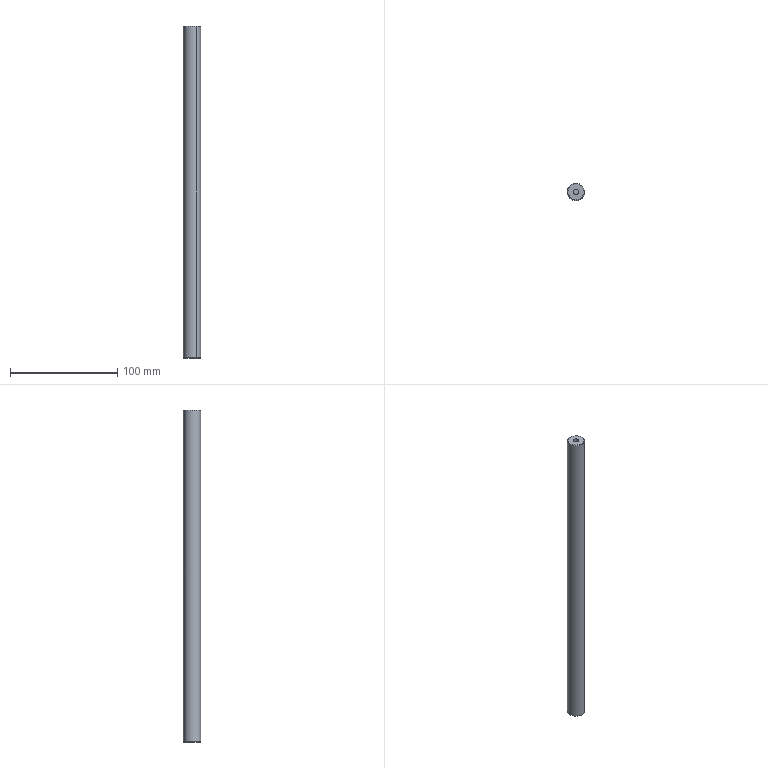Part | SolidWorks | features BaseBody 1 | 1 solid | 16 faces | box 16 x 16 x 310 mm | volume 61335 mm3 | cone 6 | cylinder 6 | plane 4 | commonest cylinder face diameters 5 x4 16 x2
STEP:
#1=CARTESIAN_POINT('',(-866.979,642.648,316.732));
#2=VERTEX_POINT('',#1);
#3=CARTESIAN_POINT('',(-869.568,632.362,316.732));
#4=VERTEX_POINT('',#3);
#5=CARTESIAN_POINT('',(-863.131,636.211,316.732));
#6=DIRECTION('',(0.,0.,1.));
#7=DIRECTION('',(-0.8583,-0.5131,0.));
#8=AXIS2_PLACEMENT_3D('',#5,#6,#7);
#9=CIRCLE('',#8,7.5);
#10=EDGE_CURVE('',#2,#4,#9,.T.);
#11=ORIENTED_EDGE('',*,*,#10,.T.);
#12=CARTESIAN_POINT('',(-869.997,632.106,317.232));
#13=VERTEX_POINT('',#12);
#14=CARTESIAN_POINT('',(-869.783,632.234,316.982));
#15=DIRECTION('',(-0.6069,-0.3628,0.7071));
#16=VECTOR('',#15,1000.);
#17=LINE('',#14,#16);
#18=EDGE_CURVE('',#4,#13,#17,.T.);
#19=ORIENTED_EDGE('',*,*,#18,.T.);
#20=CARTESIAN_POINT('',(-867.235,643.077,317.232));
#21=VERTEX_POINT('',#20);
#22=CARTESIAN_POINT('',(-863.131,636.211,317.232));
#23=DIRECTION('',(0.,0.,1.));
#24=DIRECTION('',(-0.8583,-0.5131,0.));
#25=AXIS2_PLACEMENT_3D('',#22,#23,#24);
#26=CIRCLE('',#25,8.);
#27=EDGE_CURVE('',#21,#13,#26,.T.);
#28=ORIENTED_EDGE('',*,*,#27,.F.);
#29=CARTESIAN_POINT('',(-866.979,642.648,316.732));
#30=DIRECTION('',(-0.3628,0.6069,0.7071));
#31=VECTOR('',#30,1000.);
#32=LINE('',#29,#31);
#33=EDGE_CURVE('',#2,#21,#32,.T.);
#34=ORIENTED_EDGE('',*,*,#33,.F.);
#35=EDGE_LOOP('',(#11,#19,#28,#34));
#36=FACE_OUTER_BOUND('',#35,.T.);
#37=CARTESIAN_POINT('',(-863.131,636.211,316.982));
#38=DIRECTION('',(0.,0.,1.));
#39=DIRECTION('',(-0.8583,-0.5131,0.));
#40=AXIS2_PLACEMENT_3D('',#37,#38,#39);
#41=CONICAL_SURFACE('',#40,7.75,0.7854);
#42=ADVANCED_FACE('',(#36),#41,.T.);
#43=CARTESIAN_POINT('',(-859.283,629.773,626.732));
#44=VERTEX_POINT('',#43);
#45=CARTESIAN_POINT('',(-869.568,632.362,626.732));
#46=VERTEX_POINT('',#45);
#47=CARTESIAN_POINT('',(-863.131,636.211,626.732));
#48=DIRECTION('',(0.,0.,-1.));
#49=DIRECTION('',(-0.8583,-0.5131,0.));
#50=AXIS2_PLACEMENT_3D('',#47,#48,#49);
#51=CIRCLE('',#50,7.5);
#52=EDGE_CURVE('',#44,#46,#51,.T.);
#53=ORIENTED_EDGE('',*,*,#52,.T.);
#54=CARTESIAN_POINT('',(-869.997,632.106,626.232));
#55=VERTEX_POINT('',#54);
#56=CARTESIAN_POINT('',(-869.783,632.234,626.482));
#57=DIRECTION('',(-0.6069,-0.3628,-0.7071));
#58=VECTOR('',#57,1000.);
#59=LINE('',#56,#58);
#60=EDGE_CURVE('',#46,#55,#59,.T.);
#61=ORIENTED_EDGE('',*,*,#60,.T.);
#62=CARTESIAN_POINT('',(-859.026,629.344,626.232));
#63=VERTEX_POINT('',#62);
#64=CARTESIAN_POINT('',(-863.131,636.211,626.232));
#65=DIRECTION('',(0.,0.,-1.));
#66=DIRECTION('',(-0.8583,-0.5131,0.));
#67=AXIS2_PLACEMENT_3D('',#64,#65,#66);
#68=CIRCLE('',#67,8.);
#69=EDGE_CURVE('',#63,#55,#68,.T.);
#70=ORIENTED_EDGE('',*,*,#69,.F.);
#71=CARTESIAN_POINT('',(-859.026,629.344,626.232));
#72=DIRECTION('',(-0.3628,0.6069,0.7071));
#73=VECTOR('',#72,1000.);
#74=LINE('',#71,#73);
#75=EDGE_CURVE('',#63,#44,#74,.T.);
#76=ORIENTED_EDGE('',*,*,#75,.T.);
#77=EDGE_LOOP('',(#53,#61,#70,#76));
#78=FACE_OUTER_BOUND('',#77,.T.);
#79=CARTESIAN_POINT('',(-863.131,636.211,626.482));
#80=DIRECTION('',(0.,0.,-1.));
#81=DIRECTION('',(-0.8583,-0.5131,0.));
#82=AXIS2_PLACEMENT_3D('',#79,#80,#81);
#83=CONICAL_SURFACE('',#82,7.75,0.7854);
#84=ADVANCED_FACE('',(#78),#83,.T.);
#85=CARTESIAN_POINT('',(-859.026,629.344,317.232));
#86=VERTEX_POINT('',#85);
#87=CARTESIAN_POINT('',(-859.026,629.344,317.232));
#88=DIRECTION('',(0.,0.,1.));
#89=VECTOR('',#88,1000.);
#90=LINE('',#87,#89);
#91=EDGE_CURVE('',#86,#63,#90,.T.);
#92=ORIENTED_EDGE('',*,*,#91,.F.);
#93=CARTESIAN_POINT('',(-863.131,636.211,317.232));
#94=DIRECTION('',(0.,0.,1.));
#95=DIRECTION('',(0.8583,0.5131,0.));
#96=AXIS2_PLACEMENT_3D('',#93,#94,#95);
#97=CIRCLE('',#96,8.);
#98=EDGE_CURVE('',#86,#21,#97,.T.);
#99=ORIENTED_EDGE('',*,*,#98,.T.);
#100=CARTESIAN_POINT('',(-867.235,643.077,626.232));
#101=VERTEX_POINT('',#100);
#102=CARTESIAN_POINT('',(-867.235,643.077,626.232));
#103=DIRECTION('',(0.,0.,-1.));
#104=VECTOR('',#103,1000.);
#105=LINE('',#102,#104);
#106=EDGE_CURVE('',#101,#21,#105,.T.);
#107=ORIENTED_EDGE('',*,*,#106,.F.);
#108=CARTESIAN_POINT('',(-863.131,636.211,626.232));
#109=DIRECTION('',(0.,0.,-1.));
#110=DIRECTION('',(0.8583,0.5131,0.));
#111=AXIS2_PLACEMENT_3D('',#108,#109,#110);
#112=CIRCLE('',#111,8.);
#113=EDGE_CURVE('',#101,#63,#112,.T.);
#114=ORIENTED_EDGE('',*,*,#113,.T.);
#115=EDGE_LOOP('',(#92,#99,#107,#114));
#116=FACE_OUTER_BOUND('',#115,.T.);
#117=CARTESIAN_POINT('',(-863.131,636.211,646.732));
#118=DIRECTION('',(0.,0.,-1.));
#119=DIRECTION('',(0.5131,-0.8583,0.));
#120=AXIS2_PLACEMENT_3D('',#117,#118,#119);
#121=CYLINDRICAL_SURFACE('',#120,8.);
#122=ADVANCED_FACE('',(#116),#121,.T.);
#123=ORIENTED_EDGE('',*,*,#106,.T.);
#124=ORIENTED_EDGE('',*,*,#27,.T.);
#125=CARTESIAN_POINT('',(-863.131,636.211,317.232));
#126=DIRECTION('',(0.,0.,1.));
#127=DIRECTION('',(-0.8583,-0.5131,0.));
#128=AXIS2_PLACEMENT_3D('',#125,#126,#127);
#129=CIRCLE('',#128,8.);
#130=EDGE_CURVE('',#13,#86,#129,.T.);
#131=ORIENTED_EDGE('',*,*,#130,.T.);
#132=ORIENTED_EDGE('',*,*,#91,.T.);
#133=ORIENTED_EDGE('',*,*,#69,.T.);
#134=CARTESIAN_POINT('',(-863.131,636.211,626.232));
#135=DIRECTION('',(0.,0.,-1.));
#136=DIRECTION('',(-0.8583,-0.5131,0.));
#137=AXIS2_PLACEMENT_3D('',#134,#135,#136);
#138=CIRCLE('',#137,8.);
#139=EDGE_CURVE('',#55,#101,#138,.T.);
#140=ORIENTED_EDGE('',*,*,#139,.T.);
#141=EDGE_LOOP('',(#123,#124,#131,#132,#133,#140));
#142=FACE_OUTER_BOUND('',#141,.T.);
#143=CARTESIAN_POINT('',(-863.131,636.211,646.732));
#144=DIRECTION('',(0.,0.,-1.));
#145=DIRECTION('',(0.5131,-0.8583,0.));
#146=AXIS2_PLACEMENT_3D('',#143,#144,#145);
#147=CYLINDRICAL_SURFACE('',#146,8.);
#148=ADVANCED_FACE('',(#142),#147,.T.);
#149=ORIENTED_EDGE('',*,*,#60,.F.);
#150=CARTESIAN_POINT('',(-866.979,642.648,626.732));
#151=VERTEX_POINT('',#150);
#152=CARTESIAN_POINT('',(-863.131,636.211,626.732));
#153=DIRECTION('',(0.,0.,-1.));
#154=DIRECTION('',(-0.8583,-0.5131,0.));
#155=AXIS2_PLACEMENT_3D('',#152,#153,#154);
#156=CIRCLE('',#155,7.5);
#157=EDGE_CURVE('',#46,#151,#156,.T.);
#158=ORIENTED_EDGE('',*,*,#157,.T.);
#159=CARTESIAN_POINT('',(-866.979,642.648,626.732));
#160=DIRECTION('',(-0.3628,0.6069,-0.7071));
#161=VECTOR('',#160,1000.);
#162=LINE('',#159,#161);
#163=EDGE_CURVE('',#151,#101,#162,.T.);
#164=ORIENTED_EDGE('',*,*,#163,.T.);
#165=ORIENTED_EDGE('',*,*,#139,.F.);
#166=EDGE_LOOP('',(#149,#158,#164,#165));
#167=FACE_OUTER_BOUND('',#166,.T.);
#168=CARTESIAN_POINT('',(-863.131,636.211,626.482));
#169=DIRECTION('',(0.,0.,-1.));
#170=DIRECTION('',(-0.8583,-0.5131,0.));
#171=AXIS2_PLACEMENT_3D('',#168,#169,#170);
#172=CONICAL_SURFACE('',#171,7.75,0.7854);
#173=ADVANCED_FACE('',(#167),#172,.T.);
#174=ORIENTED_EDGE('',*,*,#163,.F.);
#175=CARTESIAN_POINT('',(-863.131,636.211,626.732));
#176=DIRECTION('',(0.,0.,-1.));
#177=DIRECTION('',(0.8583,0.5131,0.));
#178=AXIS2_PLACEMENT_3D('',#175,#176,#177);
#179=CIRCLE('',#178,7.5);
#180=EDGE_CURVE('',#151,#44,#179,.T.);
#181=ORIENTED_EDGE('',*,*,#180,.T.);
#182=ORIENTED_EDGE('',*,*,#75,.F.);
#183=ORIENTED_EDGE('',*,*,#113,.F.);
#184=EDGE_LOOP('',(#174,#181,#182,#183));
#185=FACE_OUTER_BOUND('',#184,.T.);
#186=CARTESIAN_POINT('',(-863.131,636.211,626.482));
#187=DIRECTION('',(0.,0.,-1.));
#188=DIRECTION('',(-0.8583,-0.5131,0.));
#189=AXIS2_PLACEMENT_3D('',#186,#187,#188);
#190=CONICAL_SURFACE('',#189,7.75,0.7854);
#191=ADVANCED_FACE('',(#185),#190,.T.);
#192=ORIENTED_EDGE('',*,*,#52,.F.);
#193=ORIENTED_EDGE('',*,*,#180,.F.);
#194=ORIENTED_EDGE('',*,*,#157,.F.);
#195=EDGE_LOOP('',(#192,#193,#194));
#196=FACE_OUTER_BOUND('',#195,.T.);
#197=CARTESIAN_POINT('',(-861.848,634.065,626.732));
#198=VERTEX_POINT('',#197);
#199=CARTESIAN_POINT('',(-864.413,638.356,626.732));
#200=VERTEX_POINT('',#199);
#201=CARTESIAN_POINT('',(-863.131,636.211,626.732));
#202=DIRECTION('',(0.,0.,1.));
#203=DIRECTION('',(0.5131,-0.8583,0.));
#204=AXIS2_PLACEMENT_3D('',#201,#202,#203);
#205=CIRCLE('',#204,2.5);
#206=EDGE_CURVE('',#198,#200,#205,.T.);
#207=ORIENTED_EDGE('',*,*,#206,.F.);
#208=CARTESIAN_POINT('',(-863.131,636.211,626.732));
#209=DIRECTION('',(0.,0.,1.));
#210=DIRECTION('',(-0.5131,0.8583,0.));
#211=AXIS2_PLACEMENT_3D('',#208,#209,#210);
#212=CIRCLE('',#211,2.5);
#213=EDGE_CURVE('',#200,#198,#212,.T.);
#214=ORIENTED_EDGE('',*,*,#213,.F.);
#215=EDGE_LOOP('',(#207,#214));
#216=FACE_BOUND('',#215,.T.);
#217=CARTESIAN_POINT('',(-863.131,636.211,626.732));
#218=DIRECTION('',(0.,0.,1.));
#219=DIRECTION('',(-0.5131,0.8583,0.));
#220=AXIS2_PLACEMENT_3D('',#217,#218,#219);
#221=PLANE('',#220);
#222=ADVANCED_FACE('',(#196,#216),#221,.T.);
#223=CARTESIAN_POINT('',(-861.848,634.065,596.732));
#224=VERTEX_POINT('',#223);
#225=CARTESIAN_POINT('',(-864.413,638.356,596.732));
#226=VERTEX_POINT('',#225);
#227=CARTESIAN_POINT('',(-863.131,636.211,596.732));
#228=DIRECTION('',(0.,0.,-1.));
#229=DIRECTION('',(0.5131,-0.8583,0.));
#230=AXIS2_PLACEMENT_3D('',#227,#228,#229);
#231=CIRCLE('',#230,2.5);
#232=EDGE_CURVE('',#224,#226,#231,.T.);
#233=ORIENTED_EDGE('',*,*,#232,.T.);
#234=CARTESIAN_POINT('',(-864.413,638.356,596.732));
#235=DIRECTION('',(0.,0.,1.));
#236=VECTOR('',#235,1000.);
#237=LINE('',#234,#236);
#238=EDGE_CURVE('',#226,#200,#237,.T.);
#239=ORIENTED_EDGE('',*,*,#238,.T.);
#240=ORIENTED_EDGE('',*,*,#213,.T.);
#241=CARTESIAN_POINT('',(-861.848,634.065,626.732));
#242=DIRECTION('',(0.,0.,-1.));
#243=VECTOR('',#242,1000.);
#244=LINE('',#241,#243);
#245=EDGE_CURVE('',#198,#224,#244,.T.);
#246=ORIENTED_EDGE('',*,*,#245,.T.);
#247=EDGE_LOOP('',(#233,#239,#240,#246));
#248=FACE_OUTER_BOUND('',#247,.T.);
#249=CARTESIAN_POINT('',(-863.131,636.211,626.732));
#250=DIRECTION('',(0.,0.,1.));
#251=DIRECTION('',(-0.5131,0.8583,0.));
#252=AXIS2_PLACEMENT_3D('',#249,#250,#251);
#253=CYLINDRICAL_SURFACE('',#252,2.5);
#254=ADVANCED_FACE('',(#248),#253,.F.);
#255=CARTESIAN_POINT('',(-863.131,636.211,596.732));
#256=DIRECTION('',(0.,0.,-1.));
#257=DIRECTION('',(-0.5131,0.8583,0.));
#258=AXIS2_PLACEMENT_3D('',#255,#256,#257);
#259=CIRCLE('',#258,2.5);
#260=EDGE_CURVE('',#226,#224,#259,.T.);
#261=ORIENTED_EDGE('',*,*,#260,.T.);
#262=ORIENTED_EDGE('',*,*,#245,.F.);
#263=ORIENTED_EDGE('',*,*,#206,.T.);
#264=ORIENTED_EDGE('',*,*,#238,.F.);
#265=EDGE_LOOP('',(#261,#262,#263,#264));
#266=FACE_OUTER_BOUND('',#265,.T.);
#267=CARTESIAN_POINT('',(-863.131,636.211,626.732));
#268=DIRECTION('',(0.,0.,1.));
#269=DIRECTION('',(-0.5131,0.8583,0.));
#270=AXIS2_PLACEMENT_3D('',#267,#268,#269);
#271=CYLINDRICAL_SURFACE('',#270,2.5);
#272=ADVANCED_FACE('',(#266),#271,.F.);
#273=ORIENTED_EDGE('',*,*,#260,.F.);
#274=ORIENTED_EDGE('',*,*,#232,.F.);
#275=EDGE_LOOP('',(#273,#274));
#276=FACE_OUTER_BOUND('',#275,.T.);
#277=CARTESIAN_POINT('',(-863.131,636.211,596.732));
#278=DIRECTION('',(0.,0.,1.));
#279=DIRECTION('',(-0.5131,0.8583,0.));
#280=AXIS2_PLACEMENT_3D('',#277,#278,#279);
#281=PLANE('',#280);
#282=ADVANCED_FACE('',(#276),#281,.T.);
#283=ORIENTED_EDGE('',*,*,#18,.F.);
#284=CARTESIAN_POINT('',(-859.283,629.773,316.732));
#285=VERTEX_POINT('',#284);
#286=CARTESIAN_POINT('',(-863.131,636.211,316.732));
#287=DIRECTION('',(0.,0.,1.));
#288=DIRECTION('',(-0.8583,-0.5131,0.));
#289=AXIS2_PLACEMENT_3D('',#286,#287,#288);
#290=CIRCLE('',#289,7.5);
#291=EDGE_CURVE('',#4,#285,#290,.T.);
#292=ORIENTED_EDGE('',*,*,#291,.T.);
#293=CARTESIAN_POINT('',(-859.026,629.344,317.232));
#294=DIRECTION('',(-0.3628,0.6069,-0.7071));
#295=VECTOR('',#294,1000.);
#296=LINE('',#293,#295);
#297=EDGE_CURVE('',#86,#285,#296,.T.);
#298=ORIENTED_EDGE('',*,*,#297,.F.);
#299=ORIENTED_EDGE('',*,*,#130,.F.);
#300=EDGE_LOOP('',(#283,#292,#298,#299));
#301=FACE_OUTER_BOUND('',#300,.T.);
#302=CARTESIAN_POINT('',(-863.131,636.211,316.982));
#303=DIRECTION('',(0.,0.,1.));
#304=DIRECTION('',(-0.8583,-0.5131,0.));
#305=AXIS2_PLACEMENT_3D('',#302,#303,#304);
#306=CONICAL_SURFACE('',#305,7.75,0.7854);
#307=ADVANCED_FACE('',(#301),#306,.T.);
#308=ORIENTED_EDGE('',*,*,#98,.F.);
#309=ORIENTED_EDGE('',*,*,#297,.T.);
#310=CARTESIAN_POINT('',(-863.131,636.211,316.732));
#311=DIRECTION('',(0.,0.,1.));
#312=DIRECTION('',(0.8583,0.5131,0.));
#313=AXIS2_PLACEMENT_3D('',#310,#311,#312);
#314=CIRCLE('',#313,7.5);
#315=EDGE_CURVE('',#285,#2,#314,.T.);
#316=ORIENTED_EDGE('',*,*,#315,.T.);
#317=ORIENTED_EDGE('',*,*,#33,.T.);
#318=EDGE_LOOP('',(#308,#309,#316,#317));
#319=FACE_OUTER_BOUND('',#318,.T.);
#320=CARTESIAN_POINT('',(-863.131,636.211,316.982));
#321=DIRECTION('',(0.,0.,1.));
#322=DIRECTION('',(-0.8583,-0.5131,0.));
#323=AXIS2_PLACEMENT_3D('',#320,#321,#322);
#324=CONICAL_SURFACE('',#323,7.75,0.7854);
#325=ADVANCED_FACE('',(#319),#324,.T.);
#326=ORIENTED_EDGE('',*,*,#315,.F.);
#327=ORIENTED_EDGE('',*,*,#291,.F.);
#328=ORIENTED_EDGE('',*,*,#10,.F.);
#329=EDGE_LOOP('',(#326,#327,#328));
#330=FACE_OUTER_BOUND('',#329,.T.);
#331=CARTESIAN_POINT('',(-864.413,638.356,316.732));
#332=VERTEX_POINT('',#331);
#333=CARTESIAN_POINT('',(-861.848,634.065,316.732));
#334=VERTEX_POINT('',#333);
#335=CARTESIAN_POINT('',(-863.131,636.211,316.732));
#336=DIRECTION('',(0.,0.,-1.));
#337=DIRECTION('',(-0.5131,0.8583,0.));
#338=AXIS2_PLACEMENT_3D('',#335,#336,#337);
#339=CIRCLE('',#338,2.5);
#340=EDGE_CURVE('',#332,#334,#339,.T.);
#341=ORIENTED_EDGE('',*,*,#340,.F.);
#342=CARTESIAN_POINT('',(-863.131,636.211,316.732));
#343=DIRECTION('',(0.,0.,-1.));
#344=DIRECTION('',(0.5131,-0.8583,0.));
#345=AXIS2_PLACEMENT_3D('',#342,#343,#344);
#346=CIRCLE('',#345,2.5);
#347=EDGE_CURVE('',#334,#332,#346,.T.);
#348=ORIENTED_EDGE('',*,*,#347,.F.);
#349=EDGE_LOOP('',(#341,#348));
#350=FACE_BOUND('',#349,.T.);
#351=CARTESIAN_POINT('',(-863.131,636.211,316.732));
#352=DIRECTION('',(0.,0.,1.));
#353=DIRECTION('',(-0.5131,0.8583,0.));
#354=AXIS2_PLACEMENT_3D('',#351,#352,#353);
#355=PLANE('',#354);
#356=ADVANCED_FACE('',(#330,#350),#355,.F.);
#357=CARTESIAN_POINT('',(-864.413,638.356,336.732));
#358=VERTEX_POINT('',#357);
#359=CARTESIAN_POINT('',(-861.848,634.065,336.732));
#360=VERTEX_POINT('',#359);
#361=CARTESIAN_POINT('',(-863.131,636.211,336.732));
#362=DIRECTION('',(0.,0.,1.));
#363=DIRECTION('',(-0.5131,0.8583,0.));
#364=AXIS2_PLACEMENT_3D('',#361,#362,#363);
#365=CIRCLE('',#364,2.5);
#366=EDGE_CURVE('',#358,#360,#365,.T.);
#367=ORIENTED_EDGE('',*,*,#366,.T.);
#368=CARTESIAN_POINT('',(-861.848,634.065,336.732));
#369=DIRECTION('',(0.,0.,-1.));
#370=VECTOR('',#369,1000.);
#371=LINE('',#368,#370);
#372=EDGE_CURVE('',#360,#334,#371,.T.);
#373=ORIENTED_EDGE('',*,*,#372,.T.);
#374=ORIENTED_EDGE('',*,*,#347,.T.);
#375=CARTESIAN_POINT('',(-864.413,638.356,316.732));
#376=DIRECTION('',(0.,0.,1.));
#377=VECTOR('',#376,1000.);
#378=LINE('',#375,#377);
#379=EDGE_CURVE('',#332,#358,#378,.T.);
#380=ORIENTED_EDGE('',*,*,#379,.T.);
#381=EDGE_LOOP('',(#367,#373,#374,#380));
#382=FACE_OUTER_BOUND('',#381,.T.);
#383=CARTESIAN_POINT('',(-863.131,636.211,316.732));
#384=DIRECTION('',(0.,0.,-1.));
#385=DIRECTION('',(0.5131,-0.8583,0.));
#386=AXIS2_PLACEMENT_3D('',#383,#384,#385);
#387=CYLINDRICAL_SURFACE('',#386,2.5);
#388=ADVANCED_FACE('',(#382),#387,.F.);
#389=CARTESIAN_POINT('',(-863.131,636.211,336.732));
#390=DIRECTION('',(0.,0.,1.));
#391=DIRECTION('',(0.5131,-0.8583,0.));
#392=AXIS2_PLACEMENT_3D('',#389,#390,#391);
#393=CIRCLE('',#392,2.5);
#394=EDGE_CURVE('',#360,#358,#393,.T.);
#395=ORIENTED_EDGE('',*,*,#394,.T.);
#396=ORIENTED_EDGE('',*,*,#379,.F.);
#397=ORIENTED_EDGE('',*,*,#340,.T.);
#398=ORIENTED_EDGE('',*,*,#372,.F.);
#399=EDGE_LOOP('',(#395,#396,#397,#398));
#400=FACE_OUTER_BOUND('',#399,.T.);
#401=CARTESIAN_POINT('',(-863.131,636.211,316.732));
#402=DIRECTION('',(0.,0.,-1.));
#403=DIRECTION('',(0.5131,-0.8583,0.));
#404=AXIS2_PLACEMENT_3D('',#401,#402,#403);
#405=CYLINDRICAL_SURFACE('',#404,2.5);
#406=ADVANCED_FACE('',(#400),#405,.F.);
#407=ORIENTED_EDGE('',*,*,#394,.F.);
#408=ORIENTED_EDGE('',*,*,#366,.F.);
#409=EDGE_LOOP('',(#407,#408));
#410=FACE_OUTER_BOUND('',#409,.T.);
#411=CARTESIAN_POINT('',(-863.131,636.211,336.732));
#412=DIRECTION('',(0.,0.,-1.));
#413=DIRECTION('',(0.5131,-0.8583,0.));
#414=AXIS2_PLACEMENT_3D('',#411,#412,#413);
#415=PLANE('',#414);
#416=ADVANCED_FACE('',(#410),#415,.T.);
#417=CLOSED_SHELL('',(#42,#84,#122,#148,#173,#191,#222,#254,#272,#282,#307,#325,#356,#388,#406,#416));
#418=MANIFOLD_SOLID_BREP('',#417);
#419=CARTESIAN_POINT('',(0.,0.,0.));
#420=DIRECTION('',(0.,0.,1.));
#421=DIRECTION('',(1.,0.,0.));
#422=AXIS2_PLACEMENT_3D('',#419,#420,#421);
#423=(LENGTH_UNIT()NAMED_UNIT(*)SI_UNIT(.MILLI.,.METRE.));
#424=UNCERTAINTY_MEASURE_WITH_UNIT(LENGTH_MEASURE(0.00001),#423,'','');
#425=(NAMED_UNIT(*)PLANE_ANGLE_UNIT()SI_UNIT($,.RADIAN.));
#426=(NAMED_UNIT(*)SI_UNIT($,.STERADIAN.)SOLID_ANGLE_UNIT());
#427=(GEOMETRIC_REPRESENTATION_CONTEXT(3)GLOBAL_UNCERTAINTY_ASSIGNED_CONTEXT((#424))GLOBAL_UNIT_ASSIGNED_CONTEXT((#423,#425,#426))REPRESENTATION_CONTEXT('',''));
#428=ADVANCED_BREP_SHAPE_REPRESENTATION('',(#418,#422),#427);